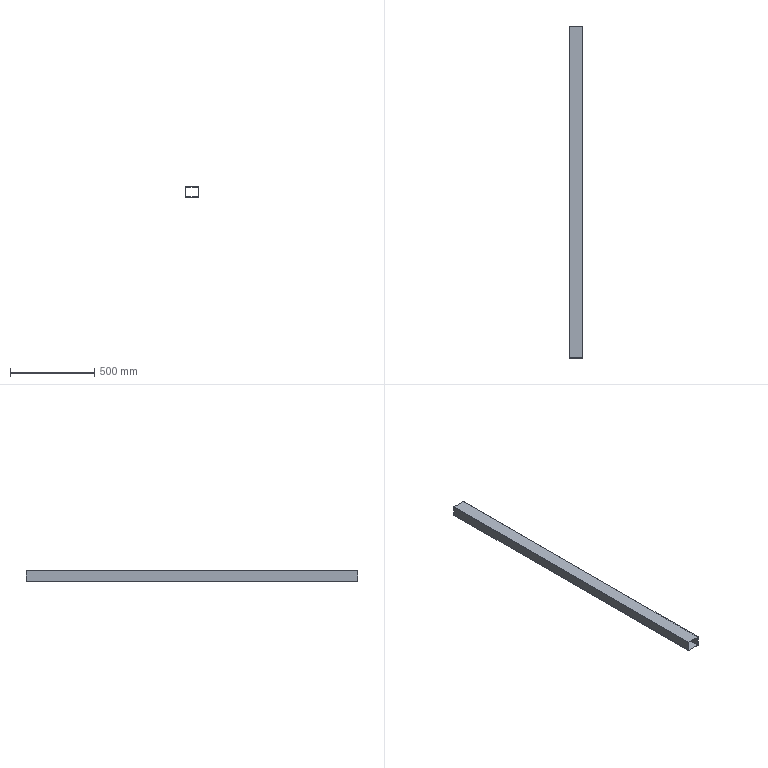Part | STEP file | Guide wheel mechanism revised.sldasm-Part-2 | 1 solid | 10 faces | box 80 x 1970 x 60 mm | volume 1583880 mm3 | plane 10
STEP:
#1=CARTESIAN_POINT('',(-485.,1970.,445.));
#2=VERTEX_POINT('',#1);
#3=CARTESIAN_POINT('',(-485.,1970.,505.));
#4=VERTEX_POINT('',#3);
#5=CARTESIAN_POINT('',(-485.,1970.,505.));
#6=DIRECTION('',(0.,0.,1.));
#7=VECTOR('',#6,1000.);
#8=LINE('',#5,#7);
#9=EDGE_CURVE('',#2,#4,#8,.T.);
#10=ORIENTED_EDGE('',*,*,#9,.T.);
#11=CARTESIAN_POINT('',(-405.,1970.,505.));
#12=VERTEX_POINT('',#11);
#13=CARTESIAN_POINT('',(-405.,1970.,505.));
#14=DIRECTION('',(1.,0.,0.));
#15=VECTOR('',#14,1000.);
#16=LINE('',#13,#15);
#17=EDGE_CURVE('',#4,#12,#16,.T.);
#18=ORIENTED_EDGE('',*,*,#17,.T.);
#19=CARTESIAN_POINT('',(-405.,1970.,445.));
#20=VERTEX_POINT('',#19);
#21=CARTESIAN_POINT('',(-405.,1970.,505.));
#22=DIRECTION('',(0.,0.,-1.));
#23=VECTOR('',#22,1000.);
#24=LINE('',#21,#23);
#25=EDGE_CURVE('',#12,#20,#24,.T.);
#26=ORIENTED_EDGE('',*,*,#25,.T.);
#27=CARTESIAN_POINT('',(-405.,1970.,445.));
#28=DIRECTION('',(-1.,0.,0.));
#29=VECTOR('',#28,1000.);
#30=LINE('',#27,#29);
#31=EDGE_CURVE('',#20,#2,#30,.T.);
#32=ORIENTED_EDGE('',*,*,#31,.T.);
#33=EDGE_LOOP('',(#10,#18,#26,#32));
#34=FACE_OUTER_BOUND('',#33,.T.);
#35=CARTESIAN_POINT('',(-408.,1970.,448.));
#36=VERTEX_POINT('',#35);
#37=CARTESIAN_POINT('',(-482.,1970.,448.));
#38=VERTEX_POINT('',#37);
#39=CARTESIAN_POINT('',(-408.,1970.,448.));
#40=DIRECTION('',(-1.,0.,0.));
#41=VECTOR('',#40,1000.);
#42=LINE('',#39,#41);
#43=EDGE_CURVE('',#36,#38,#42,.T.);
#44=ORIENTED_EDGE('',*,*,#43,.F.);
#45=CARTESIAN_POINT('',(-408.,1970.,502.));
#46=VERTEX_POINT('',#45);
#47=CARTESIAN_POINT('',(-408.,1970.,502.));
#48=DIRECTION('',(0.,0.,-1.));
#49=VECTOR('',#48,1000.);
#50=LINE('',#47,#49);
#51=EDGE_CURVE('',#46,#36,#50,.T.);
#52=ORIENTED_EDGE('',*,*,#51,.F.);
#53=CARTESIAN_POINT('',(-482.,1970.,502.));
#54=VERTEX_POINT('',#53);
#55=CARTESIAN_POINT('',(-408.,1970.,502.));
#56=DIRECTION('',(1.,0.,0.));
#57=VECTOR('',#56,1000.);
#58=LINE('',#55,#57);
#59=EDGE_CURVE('',#54,#46,#58,.T.);
#60=ORIENTED_EDGE('',*,*,#59,.F.);
#61=CARTESIAN_POINT('',(-482.,1970.,502.));
#62=DIRECTION('',(0.,0.,1.));
#63=VECTOR('',#62,1000.);
#64=LINE('',#61,#63);
#65=EDGE_CURVE('',#38,#54,#64,.T.);
#66=ORIENTED_EDGE('',*,*,#65,.F.);
#67=EDGE_LOOP('',(#44,#52,#60,#66));
#68=FACE_BOUND('',#67,.T.);
#69=CARTESIAN_POINT('',(0.,1970.,0.));
#70=DIRECTION('',(0.,1.,0.));
#71=DIRECTION('',(0.,0.,1.));
#72=AXIS2_PLACEMENT_3D('',#69,#70,#71);
#73=PLANE('',#72);
#74=ADVANCED_FACE('',(#34,#68),#73,.T.);
#75=CARTESIAN_POINT('',(-485.,0.,445.));
#76=VERTEX_POINT('',#75);
#77=CARTESIAN_POINT('',(-485.,0.,505.));
#78=VERTEX_POINT('',#77);
#79=CARTESIAN_POINT('',(-485.,0.,505.));
#80=DIRECTION('',(0.,0.,1.));
#81=VECTOR('',#80,1000.);
#82=LINE('',#79,#81);
#83=EDGE_CURVE('',#76,#78,#82,.T.);
#84=ORIENTED_EDGE('',*,*,#83,.F.);
#85=CARTESIAN_POINT('',(-405.,0.,445.));
#86=VERTEX_POINT('',#85);
#87=CARTESIAN_POINT('',(-405.,0.,445.));
#88=DIRECTION('',(-1.,0.,0.));
#89=VECTOR('',#88,1000.);
#90=LINE('',#87,#89);
#91=EDGE_CURVE('',#86,#76,#90,.T.);
#92=ORIENTED_EDGE('',*,*,#91,.F.);
#93=CARTESIAN_POINT('',(-405.,0.,505.));
#94=VERTEX_POINT('',#93);
#95=CARTESIAN_POINT('',(-405.,0.,505.));
#96=DIRECTION('',(0.,0.,-1.));
#97=VECTOR('',#96,1000.);
#98=LINE('',#95,#97);
#99=EDGE_CURVE('',#94,#86,#98,.T.);
#100=ORIENTED_EDGE('',*,*,#99,.F.);
#101=CARTESIAN_POINT('',(-405.,0.,505.));
#102=DIRECTION('',(1.,0.,0.));
#103=VECTOR('',#102,1000.);
#104=LINE('',#101,#103);
#105=EDGE_CURVE('',#78,#94,#104,.T.);
#106=ORIENTED_EDGE('',*,*,#105,.F.);
#107=EDGE_LOOP('',(#84,#92,#100,#106));
#108=FACE_OUTER_BOUND('',#107,.T.);
#109=CARTESIAN_POINT('',(-408.,0.,502.));
#110=VERTEX_POINT('',#109);
#111=CARTESIAN_POINT('',(-408.,0.,448.));
#112=VERTEX_POINT('',#111);
#113=CARTESIAN_POINT('',(-408.,0.,502.));
#114=DIRECTION('',(0.,0.,-1.));
#115=VECTOR('',#114,1000.);
#116=LINE('',#113,#115);
#117=EDGE_CURVE('',#110,#112,#116,.T.);
#118=ORIENTED_EDGE('',*,*,#117,.T.);
#119=CARTESIAN_POINT('',(-482.,0.,448.));
#120=VERTEX_POINT('',#119);
#121=CARTESIAN_POINT('',(-408.,0.,448.));
#122=DIRECTION('',(-1.,0.,0.));
#123=VECTOR('',#122,1000.);
#124=LINE('',#121,#123);
#125=EDGE_CURVE('',#112,#120,#124,.T.);
#126=ORIENTED_EDGE('',*,*,#125,.T.);
#127=CARTESIAN_POINT('',(-482.,0.,502.));
#128=VERTEX_POINT('',#127);
#129=CARTESIAN_POINT('',(-482.,0.,502.));
#130=DIRECTION('',(0.,0.,1.));
#131=VECTOR('',#130,1000.);
#132=LINE('',#129,#131);
#133=EDGE_CURVE('',#120,#128,#132,.T.);
#134=ORIENTED_EDGE('',*,*,#133,.T.);
#135=CARTESIAN_POINT('',(-408.,0.,502.));
#136=DIRECTION('',(1.,0.,0.));
#137=VECTOR('',#136,1000.);
#138=LINE('',#135,#137);
#139=EDGE_CURVE('',#128,#110,#138,.T.);
#140=ORIENTED_EDGE('',*,*,#139,.T.);
#141=EDGE_LOOP('',(#118,#126,#134,#140));
#142=FACE_BOUND('',#141,.T.);
#143=CARTESIAN_POINT('',(0.,0.,0.));
#144=DIRECTION('',(0.,1.,0.));
#145=DIRECTION('',(0.,0.,1.));
#146=AXIS2_PLACEMENT_3D('',#143,#144,#145);
#147=PLANE('',#146);
#148=ADVANCED_FACE('',(#108,#142),#147,.F.);
#149=ORIENTED_EDGE('',*,*,#83,.T.);
#150=CARTESIAN_POINT('',(-485.,1970.,505.));
#151=DIRECTION('',(0.,-1.,0.));
#152=VECTOR('',#151,1000.);
#153=LINE('',#150,#152);
#154=EDGE_CURVE('',#4,#78,#153,.T.);
#155=ORIENTED_EDGE('',*,*,#154,.F.);
#156=ORIENTED_EDGE('',*,*,#9,.F.);
#157=CARTESIAN_POINT('',(-485.,1970.,445.));
#158=DIRECTION('',(0.,-1.,0.));
#159=VECTOR('',#158,1000.);
#160=LINE('',#157,#159);
#161=EDGE_CURVE('',#2,#76,#160,.T.);
#162=ORIENTED_EDGE('',*,*,#161,.T.);
#163=EDGE_LOOP('',(#149,#155,#156,#162));
#164=FACE_OUTER_BOUND('',#163,.T.);
#165=CARTESIAN_POINT('',(-485.,1970.,505.));
#166=DIRECTION('',(1.,0.,0.));
#167=DIRECTION('',(0.,0.,-1.));
#168=AXIS2_PLACEMENT_3D('',#165,#166,#167);
#169=PLANE('',#168);
#170=ADVANCED_FACE('',(#164),#169,.F.);
#171=ORIENTED_EDGE('',*,*,#105,.T.);
#172=CARTESIAN_POINT('',(-405.,1970.,505.));
#173=DIRECTION('',(0.,-1.,0.));
#174=VECTOR('',#173,1000.);
#175=LINE('',#172,#174);
#176=EDGE_CURVE('',#12,#94,#175,.T.);
#177=ORIENTED_EDGE('',*,*,#176,.F.);
#178=ORIENTED_EDGE('',*,*,#17,.F.);
#179=ORIENTED_EDGE('',*,*,#154,.T.);
#180=EDGE_LOOP('',(#171,#177,#178,#179));
#181=FACE_OUTER_BOUND('',#180,.T.);
#182=CARTESIAN_POINT('',(-405.,1970.,505.));
#183=DIRECTION('',(0.,0.,-1.));
#184=DIRECTION('',(-1.,0.,0.));
#185=AXIS2_PLACEMENT_3D('',#182,#183,#184);
#186=PLANE('',#185);
#187=ADVANCED_FACE('',(#181),#186,.F.);
#188=ORIENTED_EDGE('',*,*,#99,.T.);
#189=CARTESIAN_POINT('',(-405.,1970.,445.));
#190=DIRECTION('',(0.,-1.,0.));
#191=VECTOR('',#190,1000.);
#192=LINE('',#189,#191);
#193=EDGE_CURVE('',#20,#86,#192,.T.);
#194=ORIENTED_EDGE('',*,*,#193,.F.);
#195=ORIENTED_EDGE('',*,*,#25,.F.);
#196=ORIENTED_EDGE('',*,*,#176,.T.);
#197=EDGE_LOOP('',(#188,#194,#195,#196));
#198=FACE_OUTER_BOUND('',#197,.T.);
#199=CARTESIAN_POINT('',(-405.,1970.,505.));
#200=DIRECTION('',(-1.,0.,0.));
#201=DIRECTION('',(0.,0.,1.));
#202=AXIS2_PLACEMENT_3D('',#199,#200,#201);
#203=PLANE('',#202);
#204=ADVANCED_FACE('',(#198),#203,.F.);
#205=ORIENTED_EDGE('',*,*,#91,.T.);
#206=ORIENTED_EDGE('',*,*,#161,.F.);
#207=ORIENTED_EDGE('',*,*,#31,.F.);
#208=ORIENTED_EDGE('',*,*,#193,.T.);
#209=EDGE_LOOP('',(#205,#206,#207,#208));
#210=FACE_OUTER_BOUND('',#209,.T.);
#211=CARTESIAN_POINT('',(-405.,1970.,445.));
#212=DIRECTION('',(0.,0.,1.));
#213=DIRECTION('',(1.,0.,0.));
#214=AXIS2_PLACEMENT_3D('',#211,#212,#213);
#215=PLANE('',#214);
#216=ADVANCED_FACE('',(#210),#215,.F.);
#217=ORIENTED_EDGE('',*,*,#117,.F.);
#218=CARTESIAN_POINT('',(-408.,1970.,502.));
#219=DIRECTION('',(0.,-1.,0.));
#220=VECTOR('',#219,1000.);
#221=LINE('',#218,#220);
#222=EDGE_CURVE('',#46,#110,#221,.T.);
#223=ORIENTED_EDGE('',*,*,#222,.F.);
#224=ORIENTED_EDGE('',*,*,#51,.T.);
#225=CARTESIAN_POINT('',(-408.,1970.,448.));
#226=DIRECTION('',(0.,-1.,0.));
#227=VECTOR('',#226,1000.);
#228=LINE('',#225,#227);
#229=EDGE_CURVE('',#36,#112,#228,.T.);
#230=ORIENTED_EDGE('',*,*,#229,.T.);
#231=EDGE_LOOP('',(#217,#223,#224,#230));
#232=FACE_OUTER_BOUND('',#231,.T.);
#233=CARTESIAN_POINT('',(-408.,1970.,502.));
#234=DIRECTION('',(-1.,0.,0.));
#235=DIRECTION('',(0.,0.,1.));
#236=AXIS2_PLACEMENT_3D('',#233,#234,#235);
#237=PLANE('',#236);
#238=ADVANCED_FACE('',(#232),#237,.T.);
#239=ORIENTED_EDGE('',*,*,#125,.F.);
#240=ORIENTED_EDGE('',*,*,#229,.F.);
#241=ORIENTED_EDGE('',*,*,#43,.T.);
#242=CARTESIAN_POINT('',(-482.,1970.,448.));
#243=DIRECTION('',(0.,-1.,0.));
#244=VECTOR('',#243,1000.);
#245=LINE('',#242,#244);
#246=EDGE_CURVE('',#38,#120,#245,.T.);
#247=ORIENTED_EDGE('',*,*,#246,.T.);
#248=EDGE_LOOP('',(#239,#240,#241,#247));
#249=FACE_OUTER_BOUND('',#248,.T.);
#250=CARTESIAN_POINT('',(-408.,1970.,448.));
#251=DIRECTION('',(0.,0.,1.));
#252=DIRECTION('',(1.,0.,0.));
#253=AXIS2_PLACEMENT_3D('',#250,#251,#252);
#254=PLANE('',#253);
#255=ADVANCED_FACE('',(#249),#254,.T.);
#256=ORIENTED_EDGE('',*,*,#133,.F.);
#257=ORIENTED_EDGE('',*,*,#246,.F.);
#258=ORIENTED_EDGE('',*,*,#65,.T.);
#259=CARTESIAN_POINT('',(-482.,1970.,502.));
#260=DIRECTION('',(0.,-1.,0.));
#261=VECTOR('',#260,1000.);
#262=LINE('',#259,#261);
#263=EDGE_CURVE('',#54,#128,#262,.T.);
#264=ORIENTED_EDGE('',*,*,#263,.T.);
#265=EDGE_LOOP('',(#256,#257,#258,#264));
#266=FACE_OUTER_BOUND('',#265,.T.);
#267=CARTESIAN_POINT('',(-482.,1970.,502.));
#268=DIRECTION('',(1.,0.,0.));
#269=DIRECTION('',(0.,0.,-1.));
#270=AXIS2_PLACEMENT_3D('',#267,#268,#269);
#271=PLANE('',#270);
#272=ADVANCED_FACE('',(#266),#271,.T.);
#273=ORIENTED_EDGE('',*,*,#139,.F.);
#274=ORIENTED_EDGE('',*,*,#263,.F.);
#275=ORIENTED_EDGE('',*,*,#59,.T.);
#276=ORIENTED_EDGE('',*,*,#222,.T.);
#277=EDGE_LOOP('',(#273,#274,#275,#276));
#278=FACE_OUTER_BOUND('',#277,.T.);
#279=CARTESIAN_POINT('',(-408.,1970.,502.));
#280=DIRECTION('',(0.,0.,-1.));
#281=DIRECTION('',(-1.,0.,0.));
#282=AXIS2_PLACEMENT_3D('',#279,#280,#281);
#283=PLANE('',#282);
#284=ADVANCED_FACE('',(#278),#283,.T.);
#285=CLOSED_SHELL('',(#74,#148,#170,#187,#204,#216,#238,#255,#272,#284));
#286=MANIFOLD_SOLID_BREP('',#285);
#287=CARTESIAN_POINT('',(0.,0.,0.));
#288=DIRECTION('',(0.,0.,1.));
#289=DIRECTION('',(1.,0.,0.));
#290=AXIS2_PLACEMENT_3D('',#287,#288,#289);
#291=(LENGTH_UNIT()NAMED_UNIT(*)SI_UNIT(.MILLI.,.METRE.));
#292=UNCERTAINTY_MEASURE_WITH_UNIT(LENGTH_MEASURE(0.00001),#291,'','');
#293=(NAMED_UNIT(*)PLANE_ANGLE_UNIT()SI_UNIT($,.RADIAN.));
#294=(NAMED_UNIT(*)SI_UNIT($,.STERADIAN.)SOLID_ANGLE_UNIT());
#295=(GEOMETRIC_REPRESENTATION_CONTEXT(3)GLOBAL_UNCERTAINTY_ASSIGNED_CONTEXT((#292))GLOBAL_UNIT_ASSIGNED_CONTEXT((#291,#293,#294))REPRESENTATION_CONTEXT('',''));
#296=ADVANCED_BREP_SHAPE_REPRESENTATION('',(#286,#290),#295);